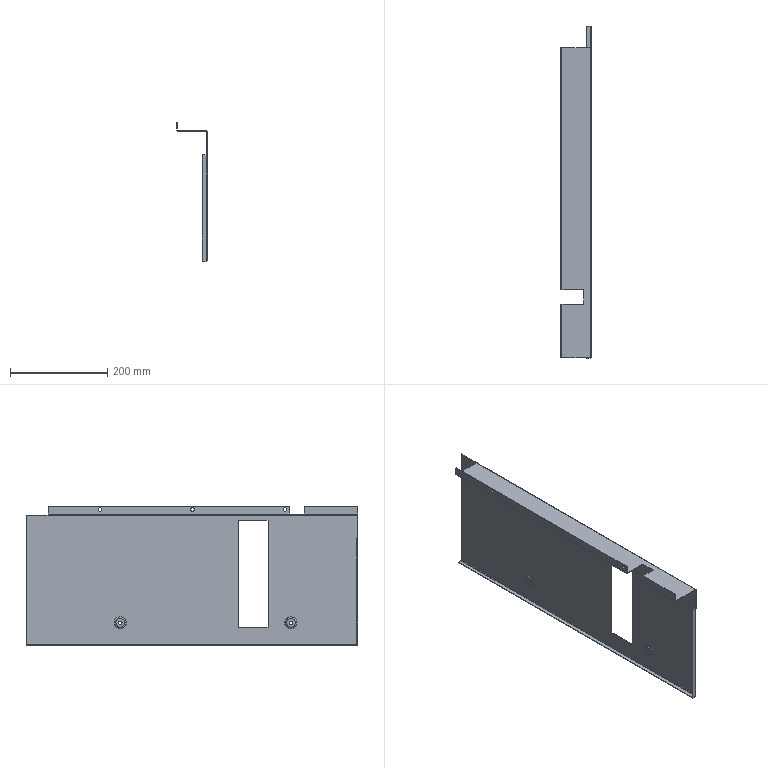Part | STEP file | 1 solid | 98 faces | box 62 x 681 x 286 mm | volume 268904 mm3 | plane 54 | cylinder 28 | torus 16 | commonest cylinder face diameters 7 x10 2 x5 4.4 x5 20 x4 22.4 x4